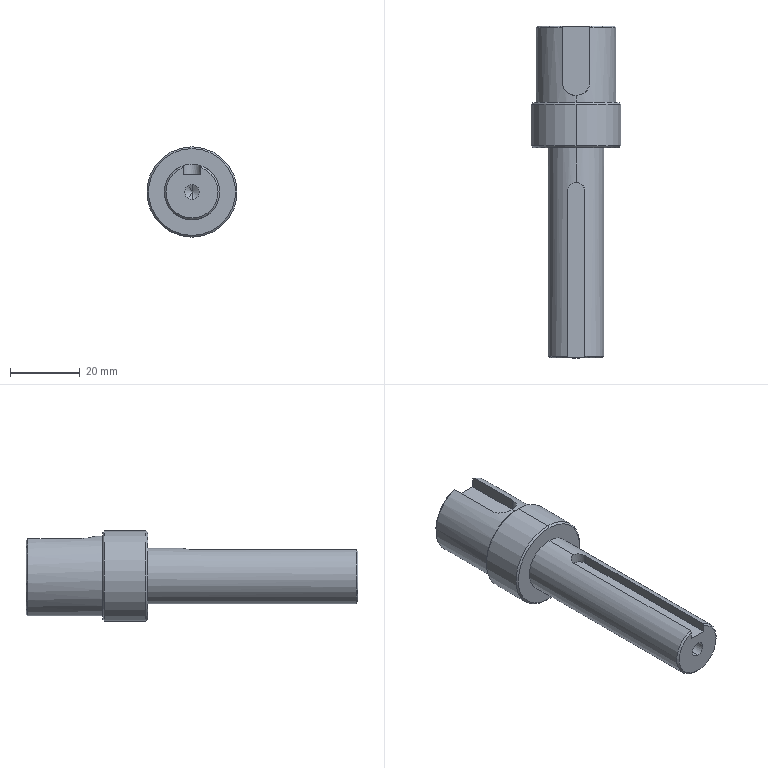Part | STEP file | ND25021-01-JDKM-20-GJ | 1 solid | 29 faces | box 26 x 95.5 x 26 mm | volume 26665 mm3 | cylinder 10 | plane 10 | cone 9 | commonest cylinder face diameters 4.2 x2 16 x2 23 x2 26 x2 5 x1 8 x1